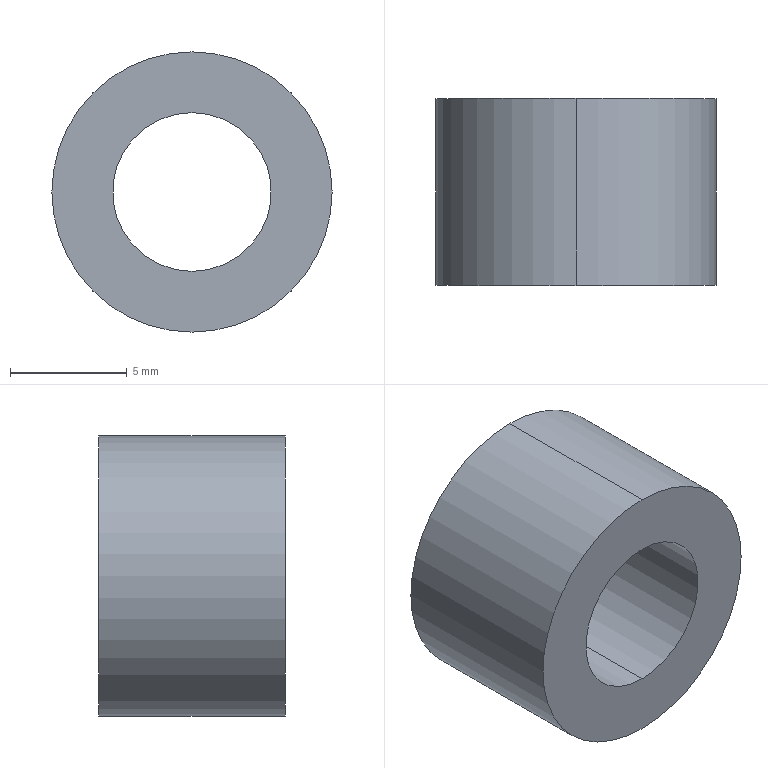Part | 1 solid | 6 faces | box 12 x 8 x 12 mm | volume 614.244 mm3 | cylinder 4 | plane 2 | commonest cylinder face diameters 6.8 x2 12 x2
STEP:
#1=CARTESIAN_POINT('',(0.,0.,-3.4));
#2=VERTEX_POINT('',#1);
#3=CARTESIAN_POINT('',(0.,0.,3.4));
#4=VERTEX_POINT('',#3);
#5=CARTESIAN_POINT('',(0.,0.,0.));
#6=DIRECTION('',(0.,1.,0.));
#7=DIRECTION('',(0.,0.,1.));
#8=AXIS2_PLACEMENT_3D('',#5,#6,#7);
#9=CIRCLE('',#8,3.4);
#10=EDGE_CURVE('',#2,#4,#9,.T.);
#11=ORIENTED_EDGE('',*,*,#10,.F.);
#12=CARTESIAN_POINT('',(0.,8.,-3.4));
#13=VERTEX_POINT('',#12);
#14=CARTESIAN_POINT('',(0.,8.,-3.4));
#15=DIRECTION('',(0.,1.,0.));
#16=VECTOR('',#15,1000.);
#17=LINE('',#14,#16);
#18=EDGE_CURVE('',#2,#13,#17,.T.);
#19=ORIENTED_EDGE('',*,*,#18,.T.);
#20=CARTESIAN_POINT('',(0.,8.,3.4));
#21=VERTEX_POINT('',#20);
#22=CARTESIAN_POINT('',(0.,8.,0.));
#23=DIRECTION('',(0.,1.,0.));
#24=DIRECTION('',(0.,0.,1.));
#25=AXIS2_PLACEMENT_3D('',#22,#23,#24);
#26=CIRCLE('',#25,3.4);
#27=EDGE_CURVE('',#13,#21,#26,.T.);
#28=ORIENTED_EDGE('',*,*,#27,.T.);
#29=CARTESIAN_POINT('',(0.,8.,3.4));
#30=DIRECTION('',(0.,1.,0.));
#31=VECTOR('',#30,1000.);
#32=LINE('',#29,#31);
#33=EDGE_CURVE('',#4,#21,#32,.T.);
#34=ORIENTED_EDGE('',*,*,#33,.F.);
#35=EDGE_LOOP('',(#11,#19,#28,#34));
#36=FACE_OUTER_BOUND('',#35,.T.);
#37=CARTESIAN_POINT('',(0.,8.,0.));
#38=DIRECTION('',(0.,1.,0.));
#39=DIRECTION('',(0.,0.,1.));
#40=AXIS2_PLACEMENT_3D('',#37,#38,#39);
#41=CYLINDRICAL_SURFACE('',#40,3.4);
#42=ADVANCED_FACE('',(#36),#41,.F.);
#43=CARTESIAN_POINT('',(0.,8.,6.));
#44=VERTEX_POINT('',#43);
#45=CARTESIAN_POINT('',(0.,8.,-6.));
#46=VERTEX_POINT('',#45);
#47=CARTESIAN_POINT('',(0.,8.,0.));
#48=DIRECTION('',(0.,1.,0.));
#49=DIRECTION('',(0.,0.,1.));
#50=AXIS2_PLACEMENT_3D('',#47,#48,#49);
#51=CIRCLE('',#50,6.);
#52=EDGE_CURVE('',#44,#46,#51,.T.);
#53=ORIENTED_EDGE('',*,*,#52,.F.);
#54=CARTESIAN_POINT('',(0.,0.,6.));
#55=VERTEX_POINT('',#54);
#56=CARTESIAN_POINT('',(0.,8.,6.));
#57=DIRECTION('',(0.,-1.,0.));
#58=VECTOR('',#57,1000.);
#59=LINE('',#56,#58);
#60=EDGE_CURVE('',#44,#55,#59,.T.);
#61=ORIENTED_EDGE('',*,*,#60,.T.);
#62=CARTESIAN_POINT('',(0.,0.,-6.));
#63=VERTEX_POINT('',#62);
#64=CARTESIAN_POINT('',(0.,0.,0.));
#65=DIRECTION('',(0.,1.,0.));
#66=DIRECTION('',(0.,0.,1.));
#67=AXIS2_PLACEMENT_3D('',#64,#65,#66);
#68=CIRCLE('',#67,6.);
#69=EDGE_CURVE('',#55,#63,#68,.T.);
#70=ORIENTED_EDGE('',*,*,#69,.T.);
#71=CARTESIAN_POINT('',(0.,8.,-6.));
#72=DIRECTION('',(0.,-1.,0.));
#73=VECTOR('',#72,1000.);
#74=LINE('',#71,#73);
#75=EDGE_CURVE('',#46,#63,#74,.T.);
#76=ORIENTED_EDGE('',*,*,#75,.F.);
#77=EDGE_LOOP('',(#53,#61,#70,#76));
#78=FACE_OUTER_BOUND('',#77,.T.);
#79=CARTESIAN_POINT('',(0.,8.,0.));
#80=DIRECTION('',(0.,-1.,0.));
#81=DIRECTION('',(0.,0.,-1.));
#82=AXIS2_PLACEMENT_3D('',#79,#80,#81);
#83=CYLINDRICAL_SURFACE('',#82,6.);
#84=ADVANCED_FACE('',(#78),#83,.T.);
#85=ORIENTED_EDGE('',*,*,#60,.F.);
#86=CARTESIAN_POINT('',(0.,8.,0.));
#87=DIRECTION('',(0.,1.,0.));
#88=DIRECTION('',(0.,0.,1.));
#89=AXIS2_PLACEMENT_3D('',#86,#87,#88);
#90=CIRCLE('',#89,6.);
#91=EDGE_CURVE('',#46,#44,#90,.T.);
#92=ORIENTED_EDGE('',*,*,#91,.F.);
#93=ORIENTED_EDGE('',*,*,#75,.T.);
#94=CARTESIAN_POINT('',(0.,0.,0.));
#95=DIRECTION('',(0.,1.,0.));
#96=DIRECTION('',(0.,0.,1.));
#97=AXIS2_PLACEMENT_3D('',#94,#95,#96);
#98=CIRCLE('',#97,6.);
#99=EDGE_CURVE('',#63,#55,#98,.T.);
#100=ORIENTED_EDGE('',*,*,#99,.T.);
#101=EDGE_LOOP('',(#85,#92,#93,#100));
#102=FACE_OUTER_BOUND('',#101,.T.);
#103=CARTESIAN_POINT('',(0.,8.,0.));
#104=DIRECTION('',(0.,-1.,0.));
#105=DIRECTION('',(0.,0.,-1.));
#106=AXIS2_PLACEMENT_3D('',#103,#104,#105);
#107=CYLINDRICAL_SURFACE('',#106,6.);
#108=ADVANCED_FACE('',(#102),#107,.T.);
#109=CARTESIAN_POINT('',(0.,8.,0.));
#110=DIRECTION('',(0.,1.,0.));
#111=DIRECTION('',(0.,0.,1.));
#112=AXIS2_PLACEMENT_3D('',#109,#110,#111);
#113=CIRCLE('',#112,3.4);
#114=EDGE_CURVE('',#21,#13,#113,.T.);
#115=ORIENTED_EDGE('',*,*,#114,.F.);
#116=ORIENTED_EDGE('',*,*,#27,.F.);
#117=EDGE_LOOP('',(#115,#116));
#118=FACE_BOUND('',#117,.T.);
#119=ORIENTED_EDGE('',*,*,#91,.T.);
#120=ORIENTED_EDGE('',*,*,#52,.T.);
#121=EDGE_LOOP('',(#119,#120));
#122=FACE_OUTER_BOUND('',#121,.T.);
#123=CARTESIAN_POINT('',(0.,8.,0.));
#124=DIRECTION('',(0.,1.,0.));
#125=DIRECTION('',(0.,0.,1.));
#126=AXIS2_PLACEMENT_3D('',#123,#124,#125);
#127=PLANE('',#126);
#128=ADVANCED_FACE('',(#118,#122),#127,.T.);
#129=CARTESIAN_POINT('',(0.,0.,0.));
#130=DIRECTION('',(0.,1.,0.));
#131=DIRECTION('',(0.,0.,1.));
#132=AXIS2_PLACEMENT_3D('',#129,#130,#131);
#133=CIRCLE('',#132,3.4);
#134=EDGE_CURVE('',#4,#2,#133,.T.);
#135=ORIENTED_EDGE('',*,*,#134,.T.);
#136=ORIENTED_EDGE('',*,*,#10,.T.);
#137=EDGE_LOOP('',(#135,#136));
#138=FACE_BOUND('',#137,.T.);
#139=ORIENTED_EDGE('',*,*,#99,.F.);
#140=ORIENTED_EDGE('',*,*,#69,.F.);
#141=EDGE_LOOP('',(#139,#140));
#142=FACE_OUTER_BOUND('',#141,.T.);
#143=CARTESIAN_POINT('',(0.,0.,0.));
#144=DIRECTION('',(0.,1.,0.));
#145=DIRECTION('',(0.,0.,1.));
#146=AXIS2_PLACEMENT_3D('',#143,#144,#145);
#147=PLANE('',#146);
#148=ADVANCED_FACE('',(#138,#142),#147,.F.);
#149=ORIENTED_EDGE('',*,*,#18,.F.);
#150=ORIENTED_EDGE('',*,*,#134,.F.);
#151=ORIENTED_EDGE('',*,*,#33,.T.);
#152=ORIENTED_EDGE('',*,*,#114,.T.);
#153=EDGE_LOOP('',(#149,#150,#151,#152));
#154=FACE_OUTER_BOUND('',#153,.T.);
#155=CARTESIAN_POINT('',(0.,8.,0.));
#156=DIRECTION('',(0.,1.,0.));
#157=DIRECTION('',(0.,0.,1.));
#158=AXIS2_PLACEMENT_3D('',#155,#156,#157);
#159=CYLINDRICAL_SURFACE('',#158,3.4);
#160=ADVANCED_FACE('',(#154),#159,.F.);
#161=CLOSED_SHELL('',(#42,#84,#108,#128,#148,#160));
#162=MANIFOLD_SOLID_BREP('',#161);
#163=CARTESIAN_POINT('',(0.,0.,0.));
#164=DIRECTION('',(0.,0.,1.));
#165=DIRECTION('',(1.,0.,0.));
#166=AXIS2_PLACEMENT_3D('',#163,#164,#165);
#167=(LENGTH_UNIT()NAMED_UNIT(*)SI_UNIT(.MILLI.,.METRE.));
#168=UNCERTAINTY_MEASURE_WITH_UNIT(LENGTH_MEASURE(0.00001),#167,'','');
#169=(NAMED_UNIT(*)PLANE_ANGLE_UNIT()SI_UNIT($,.RADIAN.));
#170=(NAMED_UNIT(*)SI_UNIT($,.STERADIAN.)SOLID_ANGLE_UNIT());
#171=(GEOMETRIC_REPRESENTATION_CONTEXT(3)GLOBAL_UNCERTAINTY_ASSIGNED_CONTEXT((#168))GLOBAL_UNIT_ASSIGNED_CONTEXT((#167,#169,#170))REPRESENTATION_CONTEXT('',''));
#172=ADVANCED_BREP_SHAPE_REPRESENTATION('',(#162,#166),#171);